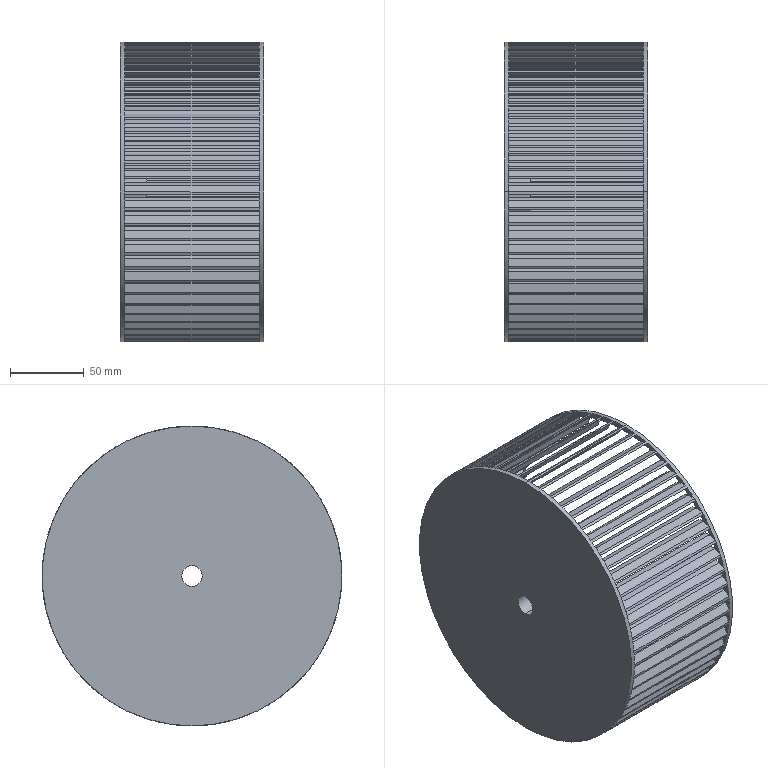Part | STEP file | 8-inch fan wheel | 1 solid | 494 faces | box 97 x 203 x 203 mm | volume 178976 mm3 | plane 484 | cylinder 10 | commonest cylinder face diameters 203 x4 14 x2 26 x2 196 x2